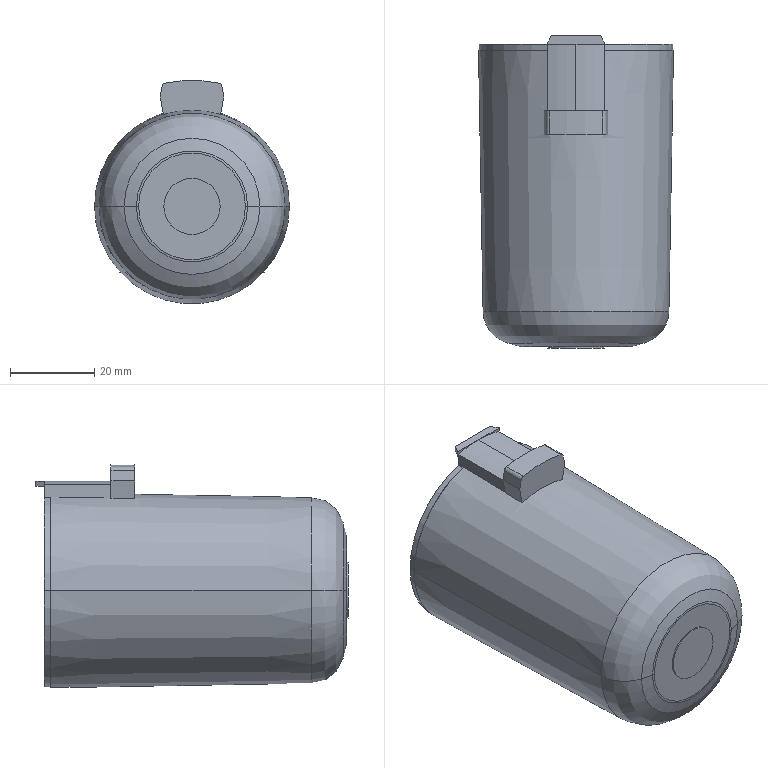Part | SolidWorks | features BaseBody 1 | 1 solid | 36 faces | box 46.4 x 74.3 x 53.2 mm | volume 114523 mm3 | plane 18 | cylinder 10 | torus 4 | cone 4 | commonest cylinder face diameters 46 x3 2 x2 13.4 x2 51.98 x2 60 x1
STEP:
#1=CARTESIAN_POINT('',(6.7,-103.95,0.));
#2=VERTEX_POINT('',#1);
#3=CARTESIAN_POINT('',(-6.7,-103.95,0.));
#4=VERTEX_POINT('',#3);
#5=CARTESIAN_POINT('',(0.,-103.95,0.));
#6=DIRECTION('',(0.,-1.,0.));
#7=DIRECTION('',(1.,0.,0.));
#8=AXIS2_PLACEMENT_3D('',#5,#6,#7);
#9=CIRCLE('',#8,6.7);
#10=EDGE_CURVE('',#2,#4,#9,.T.);
#11=ORIENTED_EDGE('',*,*,#10,.T.);
#12=CARTESIAN_POINT('',(-6.7,-104.3,0.));
#13=VERTEX_POINT('',#12);
#14=CARTESIAN_POINT('',(-6.7,-104.3,0.));
#15=DIRECTION('',(0.,-1.,0.));
#16=VECTOR('',#15,1000.);
#17=LINE('',#14,#16);
#18=EDGE_CURVE('',#4,#13,#17,.T.);
#19=ORIENTED_EDGE('',*,*,#18,.T.);
#20=CARTESIAN_POINT('',(6.7,-104.3,0.));
#21=VERTEX_POINT('',#20);
#22=CARTESIAN_POINT('',(0.,-104.3,0.));
#23=DIRECTION('',(0.,-1.,0.));
#24=DIRECTION('',(1.,0.,0.));
#25=AXIS2_PLACEMENT_3D('',#22,#23,#24);
#26=CIRCLE('',#25,6.7);
#27=EDGE_CURVE('',#21,#13,#26,.T.);
#28=ORIENTED_EDGE('',*,*,#27,.F.);
#29=CARTESIAN_POINT('',(6.7,-104.3,0.));
#30=DIRECTION('',(0.,-1.,0.));
#31=VECTOR('',#30,1000.);
#32=LINE('',#29,#31);
#33=EDGE_CURVE('',#2,#21,#32,.T.);
#34=ORIENTED_EDGE('',*,*,#33,.F.);
#35=EDGE_LOOP('',(#11,#19,#28,#34));
#36=FACE_OUTER_BOUND('',#35,.T.);
#37=CARTESIAN_POINT('',(0.,-104.3,0.));
#38=DIRECTION('',(0.,-1.,0.));
#39=DIRECTION('',(1.,0.,0.));
#40=AXIS2_PLACEMENT_3D('',#37,#38,#39);
#41=CYLINDRICAL_SURFACE('',#40,6.7);
#42=ADVANCED_FACE('',(#36),#41,.T.);
#43=CARTESIAN_POINT('',(13.254,-103.882,0.));
#44=VERTEX_POINT('',#43);
#45=CARTESIAN_POINT('',(-13.254,-103.882,0.));
#46=VERTEX_POINT('',#45);
#47=CARTESIAN_POINT('',(0.,-103.882,0.));
#48=DIRECTION('',(0.,-1.,0.));
#49=DIRECTION('',(1.,0.,0.));
#50=AXIS2_PLACEMENT_3D('',#47,#48,#49);
#51=CIRCLE('',#50,13.254);
#52=EDGE_CURVE('',#44,#46,#51,.T.);
#53=ORIENTED_EDGE('',*,*,#52,.T.);
#54=CARTESIAN_POINT('',(-12.737,-103.95,0.));
#55=VERTEX_POINT('',#54);
#56=CARTESIAN_POINT('',(-12.737,-101.95,0.));
#57=DIRECTION('',(0.,0.,1.));
#58=DIRECTION('',(1.,0.,0.));
#59=AXIS2_PLACEMENT_3D('',#56,#57,#58);
#60=CIRCLE('',#59,2.);
#61=EDGE_CURVE('',#46,#55,#60,.T.);
#62=ORIENTED_EDGE('',*,*,#61,.T.);
#63=CARTESIAN_POINT('',(12.737,-103.95,0.));
#64=VERTEX_POINT('',#63);
#65=CARTESIAN_POINT('',(0.,-103.95,0.));
#66=DIRECTION('',(0.,-1.,0.));
#67=DIRECTION('',(1.,0.,0.));
#68=AXIS2_PLACEMENT_3D('',#65,#66,#67);
#69=CIRCLE('',#68,12.737);
#70=EDGE_CURVE('',#64,#55,#69,.T.);
#71=ORIENTED_EDGE('',*,*,#70,.F.);
#72=CARTESIAN_POINT('',(12.737,-101.95,0.));
#73=DIRECTION('',(0.,0.,-1.));
#74=DIRECTION('',(-1.,0.,0.));
#75=AXIS2_PLACEMENT_3D('',#72,#73,#74);
#76=CIRCLE('',#75,2.);
#77=EDGE_CURVE('',#44,#64,#76,.T.);
#78=ORIENTED_EDGE('',*,*,#77,.F.);
#79=EDGE_LOOP('',(#53,#62,#71,#78));
#80=FACE_OUTER_BOUND('',#79,.T.);
#81=CARTESIAN_POINT('',(0.,-101.95,0.));
#82=DIRECTION('',(0.,-1.,0.));
#83=DIRECTION('',(1.,0.,0.));
#84=AXIS2_PLACEMENT_3D('',#81,#82,#83);
#85=TOROIDAL_SURFACE('',#84,12.737,2.);
#86=ADVANCED_FACE('',(#80),#85,.T.);
#87=ORIENTED_EDGE('',*,*,#52,.F.);
#88=CARTESIAN_POINT('',(16.19,-103.095,0.));
#89=VERTEX_POINT('',#88);
#90=CARTESIAN_POINT('',(16.19,-103.095,0.));
#91=DIRECTION('',(0.9659,0.2588,0.));
#92=VECTOR('',#91,1000.);
#93=LINE('',#90,#92);
#94=EDGE_CURVE('',#44,#89,#93,.T.);
#95=ORIENTED_EDGE('',*,*,#94,.T.);
#96=CARTESIAN_POINT('',(-16.19,-103.095,0.));
#97=VERTEX_POINT('',#96);
#98=CARTESIAN_POINT('',(0.,-103.095,0.));
#99=DIRECTION('',(0.,-1.,0.));
#100=DIRECTION('',(1.,0.,0.));
#101=AXIS2_PLACEMENT_3D('',#98,#99,#100);
#102=CIRCLE('',#101,16.19);
#103=EDGE_CURVE('',#89,#97,#102,.T.);
#104=ORIENTED_EDGE('',*,*,#103,.T.);
#105=CARTESIAN_POINT('',(-16.19,-103.095,0.));
#106=DIRECTION('',(-0.9659,0.2588,0.));
#107=VECTOR('',#106,1000.);
#108=LINE('',#105,#107);
#109=EDGE_CURVE('',#46,#97,#108,.T.);
#110=ORIENTED_EDGE('',*,*,#109,.F.);
#111=EDGE_LOOP('',(#87,#95,#104,#110));
#112=FACE_OUTER_BOUND('',#111,.T.);
#113=CARTESIAN_POINT('',(0.,-103.095,0.));
#114=DIRECTION('',(0.,1.,0.));
#115=DIRECTION('',(-1.,0.,0.));
#116=AXIS2_PLACEMENT_3D('',#113,#114,#115);
#117=CONICAL_SURFACE('',#116,16.19,1.309);
#118=ADVANCED_FACE('',(#112),#117,.T.);
#119=CARTESIAN_POINT('',(22.119,-95.507,0.));
#120=VERTEX_POINT('',#119);
#121=CARTESIAN_POINT('',(-22.119,-95.507,0.));
#122=VERTEX_POINT('',#121);
#123=CARTESIAN_POINT('',(0.,-95.507,0.));
#124=DIRECTION('',(0.,-1.,0.));
#125=DIRECTION('',(1.,0.,0.));
#126=AXIS2_PLACEMENT_3D('',#123,#124,#125);
#127=CIRCLE('',#126,22.119);
#128=EDGE_CURVE('',#120,#122,#127,.T.);
#129=ORIENTED_EDGE('',*,*,#128,.T.);
#130=CARTESIAN_POINT('',(-14.12,-95.368,0.));
#131=DIRECTION('',(0.,0.,1.));
#132=DIRECTION('',(1.,0.,0.));
#133=AXIS2_PLACEMENT_3D('',#130,#131,#132);
#134=CIRCLE('',#133,8.);
#135=EDGE_CURVE('',#122,#97,#134,.T.);
#136=ORIENTED_EDGE('',*,*,#135,.T.);
#137=ORIENTED_EDGE('',*,*,#103,.F.);
#138=CARTESIAN_POINT('',(14.12,-95.368,0.));
#139=DIRECTION('',(0.,0.,-1.));
#140=DIRECTION('',(-1.,0.,0.));
#141=AXIS2_PLACEMENT_3D('',#138,#139,#140);
#142=CIRCLE('',#141,8.);
#143=EDGE_CURVE('',#120,#89,#142,.T.);
#144=ORIENTED_EDGE('',*,*,#143,.F.);
#145=EDGE_LOOP('',(#129,#136,#137,#144));
#146=FACE_OUTER_BOUND('',#145,.T.);
#147=CARTESIAN_POINT('',(0.,-95.368,0.));
#148=DIRECTION('',(0.,-1.,0.));
#149=DIRECTION('',(1.,0.,0.));
#150=AXIS2_PLACEMENT_3D('',#147,#148,#149);
#151=TOROIDAL_SURFACE('',#150,14.12,8.);
#152=ADVANCED_FACE('',(#146),#151,.T.);
#153=ORIENTED_EDGE('',*,*,#128,.F.);
#154=CARTESIAN_POINT('',(23.2,-33.55,0.));
#155=VERTEX_POINT('',#154);
#156=CARTESIAN_POINT('',(23.2,-33.55,0.));
#157=DIRECTION('',(0.01745,0.9998,0.));
#158=VECTOR('',#157,1000.);
#159=LINE('',#156,#158);
#160=EDGE_CURVE('',#120,#155,#159,.T.);
#161=ORIENTED_EDGE('',*,*,#160,.T.);
#162=CARTESIAN_POINT('',(6.7,-33.55,22.211));
#163=VERTEX_POINT('',#162);
#164=CARTESIAN_POINT('',(0.,-33.55,0.));
#165=DIRECTION('',(0.,-1.,0.));
#166=DIRECTION('',(-0.2888,0.,0.9574));
#167=AXIS2_PLACEMENT_3D('',#164,#165,#166);
#168=CIRCLE('',#167,23.2);
#169=EDGE_CURVE('',#155,#163,#168,.T.);
#170=ORIENTED_EDGE('',*,*,#169,.T.);
#171=CARTESIAN_POINT('',(6.7,-47.86,21.95));
#172=VERTEX_POINT('',#171);
#173=CARTESIAN_POINT('',(6.7,-33.55,22.211));
#174=CARTESIAN_POINT('',(6.7,-38.32,22.125));
#175=CARTESIAN_POINT('',(6.7,-43.09,22.038));
#176=CARTESIAN_POINT('',(6.7,-47.86,21.95));
#177=B_SPLINE_CURVE_WITH_KNOTS('',3,(#173,#174,#175,#176),.UNSPECIFIED.,.F.,.F.,(4,4),(20.424,34.736),.UNSPECIFIED.);
#178=EDGE_CURVE('',#163,#172,#177,.T.);
#179=ORIENTED_EDGE('',*,*,#178,.T.);
#180=CARTESIAN_POINT('',(6.8,-47.86,21.92));
#181=VERTEX_POINT('',#180);
#182=CARTESIAN_POINT('',(0.,-47.86,0.));
#183=DIRECTION('',(0.,1.,0.));
#184=DIRECTION('',(0.2919,0.,0.9564));
#185=AXIS2_PLACEMENT_3D('',#182,#183,#184);
#186=CIRCLE('',#185,22.95);
#187=EDGE_CURVE('',#172,#181,#186,.T.);
#188=ORIENTED_EDGE('',*,*,#187,.T.);
#189=CARTESIAN_POINT('',(6.782,-53.5,21.822));
#190=VERTEX_POINT('',#189);
#191=CARTESIAN_POINT('',(6.782,-53.5,21.822));
#192=CARTESIAN_POINT('',(6.788,-51.62,21.855));
#193=CARTESIAN_POINT('',(6.794,-49.74,21.887));
#194=CARTESIAN_POINT('',(6.8,-47.86,21.92));
#195=B_SPLINE_CURVE_WITH_KNOTS('',3,(#191,#192,#193,#194),.UNSPECIFIED.,.F.,.F.,(4,4),(0.0002,5.641),.UNSPECIFIED.);
#196=EDGE_CURVE('',#190,#181,#195,.T.);
#197=ORIENTED_EDGE('',*,*,#196,.F.);
#198=CARTESIAN_POINT('',(-6.782,-53.5,21.822));
#199=VERTEX_POINT('',#198);
#200=CARTESIAN_POINT('',(0.,-53.5,0.));
#201=DIRECTION('',(0.,1.,0.));
#202=DIRECTION('',(-0.2968,0.,0.9549));
#203=AXIS2_PLACEMENT_3D('',#200,#201,#202);
#204=CIRCLE('',#203,22.852);
#205=EDGE_CURVE('',#199,#190,#204,.T.);
#206=ORIENTED_EDGE('',*,*,#205,.F.);
#207=CARTESIAN_POINT('',(-6.8,-47.86,21.92));
#208=VERTEX_POINT('',#207);
#209=CARTESIAN_POINT('',(-6.8,-47.86,21.92));
#210=CARTESIAN_POINT('',(-6.794,-49.74,21.887));
#211=CARTESIAN_POINT('',(-6.788,-51.62,21.855));
#212=CARTESIAN_POINT('',(-6.782,-53.5,21.822));
#213=B_SPLINE_CURVE_WITH_KNOTS('',3,(#209,#210,#211,#212),.UNSPECIFIED.,.F.,.F.,(4,4),(0.0002,5.641),.UNSPECIFIED.);
#214=EDGE_CURVE('',#208,#199,#213,.T.);
#215=ORIENTED_EDGE('',*,*,#214,.F.);
#216=CARTESIAN_POINT('',(-6.7,-47.86,21.95));
#217=VERTEX_POINT('',#216);
#218=CARTESIAN_POINT('',(0.,-47.86,0.));
#219=DIRECTION('',(0.,1.,0.));
#220=DIRECTION('',(-0.2963,0.,0.9551));
#221=AXIS2_PLACEMENT_3D('',#218,#219,#220);
#222=CIRCLE('',#221,22.95);
#223=EDGE_CURVE('',#208,#217,#222,.T.);
#224=ORIENTED_EDGE('',*,*,#223,.T.);
#225=CARTESIAN_POINT('',(-6.7,-33.55,22.211));
#226=VERTEX_POINT('',#225);
#227=CARTESIAN_POINT('',(-6.7,-47.86,21.95));
#228=CARTESIAN_POINT('',(-6.7,-43.09,22.038));
#229=CARTESIAN_POINT('',(-6.7,-38.32,22.125));
#230=CARTESIAN_POINT('',(-6.7,-33.55,22.211));
#231=B_SPLINE_CURVE_WITH_KNOTS('',3,(#227,#228,#229,#230),.UNSPECIFIED.,.F.,.F.,(4,4),(26.064,40.377),.UNSPECIFIED.);
#232=EDGE_CURVE('',#217,#226,#231,.T.);
#233=ORIENTED_EDGE('',*,*,#232,.T.);
#234=CARTESIAN_POINT('',(-23.2,-33.55,0.));
#235=VERTEX_POINT('',#234);
#236=CARTESIAN_POINT('',(0.,-33.55,0.));
#237=DIRECTION('',(0.,-1.,0.));
#238=DIRECTION('',(-0.2888,0.,0.9574));
#239=AXIS2_PLACEMENT_3D('',#236,#237,#238);
#240=CIRCLE('',#239,23.2);
#241=EDGE_CURVE('',#226,#235,#240,.T.);
#242=ORIENTED_EDGE('',*,*,#241,.T.);
#243=CARTESIAN_POINT('',(-23.2,-33.55,0.));
#244=DIRECTION('',(-0.01745,0.9998,0.));
#245=VECTOR('',#244,1000.);
#246=LINE('',#243,#245);
#247=EDGE_CURVE('',#122,#235,#246,.T.);
#248=ORIENTED_EDGE('',*,*,#247,.F.);
#249=EDGE_LOOP('',(#153,#161,#170,#179,#188,#197,#206,#215,#224,#233,#242,#248));
#250=FACE_OUTER_BOUND('',#249,.T.);
#251=CARTESIAN_POINT('',(0.,-33.55,0.));
#252=DIRECTION('',(0.,1.,0.));
#253=DIRECTION('',(-1.,0.,0.));
#254=AXIS2_PLACEMENT_3D('',#251,#252,#253);
#255=CONICAL_SURFACE('',#254,23.2,0.01745);
#256=ADVANCED_FACE('',(#250),#255,.T.);
#257=CARTESIAN_POINT('',(0.,-47.86,25.99));
#258=VERTEX_POINT('',#257);
#259=CARTESIAN_POINT('',(-6.7,-47.86,25.112));
#260=VERTEX_POINT('',#259);
#261=CARTESIAN_POINT('',(0.,-47.86,0.));
#262=DIRECTION('',(0.,-1.,0.));
#263=DIRECTION('',(0.2578,0.,0.9662));
#264=AXIS2_PLACEMENT_3D('',#261,#262,#263);
#265=CIRCLE('',#264,25.99);
#266=EDGE_CURVE('',#258,#260,#265,.T.);
#267=ORIENTED_EDGE('',*,*,#266,.F.);
#268=CARTESIAN_POINT('',(0.,-32.,25.99));
#269=VERTEX_POINT('',#268);
#270=CARTESIAN_POINT('',(0.,-53.5,25.99));
#271=DIRECTION('',(0.,1.,0.));
#272=VECTOR('',#271,1000.);
#273=LINE('',#270,#272);
#274=EDGE_CURVE('',#258,#269,#273,.T.);
#275=ORIENTED_EDGE('',*,*,#274,.T.);
#276=CARTESIAN_POINT('',(-6.7,-32.,25.112));
#277=VERTEX_POINT('',#276);
#278=CARTESIAN_POINT('',(0.,-32.,0.));
#279=DIRECTION('',(0.,1.,0.));
#280=DIRECTION('',(-0.2578,0.,0.9662));
#281=AXIS2_PLACEMENT_3D('',#278,#279,#280);
#282=CIRCLE('',#281,25.99);
#283=EDGE_CURVE('',#277,#269,#282,.T.);
#284=ORIENTED_EDGE('',*,*,#283,.F.);
#285=CARTESIAN_POINT('',(-6.7,-47.86,25.112));
#286=DIRECTION('',(0.,1.,0.));
#287=VECTOR('',#286,1000.);
#288=LINE('',#285,#287);
#289=EDGE_CURVE('',#260,#277,#288,.T.);
#290=ORIENTED_EDGE('',*,*,#289,.F.);
#291=EDGE_LOOP('',(#267,#275,#284,#290));
#292=FACE_OUTER_BOUND('',#291,.T.);
#293=CARTESIAN_POINT('',(0.,-53.5,0.));
#294=DIRECTION('',(0.,1.,0.));
#295=DIRECTION('',(0.,0.,1.));
#296=AXIS2_PLACEMENT_3D('',#293,#294,#295);
#297=CYLINDRICAL_SURFACE('',#296,25.99);
#298=ADVANCED_FACE('',(#292),#297,.T.);
#299=CARTESIAN_POINT('',(-6.7,-32.,22.002));
#300=VERTEX_POINT('',#299);
#301=CARTESIAN_POINT('',(-23.,-32.,0.));
#302=VERTEX_POINT('',#301);
#303=CARTESIAN_POINT('',(0.,-32.,0.));
#304=DIRECTION('',(0.,-1.,0.));
#305=DIRECTION('',(-0.2913,0.,0.9566));
#306=AXIS2_PLACEMENT_3D('',#303,#304,#305);
#307=CIRCLE('',#306,23.);
#308=EDGE_CURVE('',#300,#302,#307,.T.);
#309=ORIENTED_EDGE('',*,*,#308,.T.);
#310=CARTESIAN_POINT('',(-23.,-33.55,0.));
#311=VERTEX_POINT('',#310);
#312=CARTESIAN_POINT('',(-23.,-104.3,0.));
#313=DIRECTION('',(0.,-1.,0.));
#314=VECTOR('',#313,1000.);
#315=LINE('',#312,#314);
#316=EDGE_CURVE('',#302,#311,#315,.T.);
#317=ORIENTED_EDGE('',*,*,#316,.T.);
#318=CARTESIAN_POINT('',(-6.7,-33.55,22.002));
#319=VERTEX_POINT('',#318);
#320=CARTESIAN_POINT('',(0.,-33.55,0.));
#321=DIRECTION('',(0.,-1.,0.));
#322=DIRECTION('',(-0.2913,0.,0.9566));
#323=AXIS2_PLACEMENT_3D('',#320,#321,#322);
#324=CIRCLE('',#323,23.);
#325=EDGE_CURVE('',#319,#311,#324,.T.);
#326=ORIENTED_EDGE('',*,*,#325,.F.);
#327=CARTESIAN_POINT('',(-6.7,-33.55,22.002));
#328=DIRECTION('',(0.,1.,0.));
#329=VECTOR('',#328,1000.);
#330=LINE('',#327,#329);
#331=EDGE_CURVE('',#319,#300,#330,.T.);
#332=ORIENTED_EDGE('',*,*,#331,.T.);
#333=EDGE_LOOP('',(#309,#317,#326,#332));
#334=FACE_OUTER_BOUND('',#333,.T.);
#335=CARTESIAN_POINT('',(0.,-104.3,0.));
#336=DIRECTION('',(0.,-1.,0.));
#337=DIRECTION('',(1.,0.,0.));
#338=AXIS2_PLACEMENT_3D('',#335,#336,#337);
#339=CYLINDRICAL_SURFACE('',#338,23.);
#340=ADVANCED_FACE('',(#334),#339,.T.);
#341=ORIENTED_EDGE('',*,*,#316,.F.);
#342=CARTESIAN_POINT('',(23.,-32.,0.));
#343=VERTEX_POINT('',#342);
#344=CARTESIAN_POINT('',(0.,-32.,0.));
#345=DIRECTION('',(0.,-1.,0.));
#346=DIRECTION('',(-0.2913,0.,0.9566));
#347=AXIS2_PLACEMENT_3D('',#344,#345,#346);
#348=CIRCLE('',#347,23.);
#349=EDGE_CURVE('',#302,#343,#348,.T.);
#350=ORIENTED_EDGE('',*,*,#349,.T.);
#351=CARTESIAN_POINT('',(23.,-33.55,0.));
#352=VERTEX_POINT('',#351);
#353=CARTESIAN_POINT('',(23.,-104.3,0.));
#354=DIRECTION('',(0.,-1.,0.));
#355=VECTOR('',#354,1000.);
#356=LINE('',#353,#355);
#357=EDGE_CURVE('',#343,#352,#356,.T.);
#358=ORIENTED_EDGE('',*,*,#357,.T.);
#359=CARTESIAN_POINT('',(0.,-33.55,0.));
#360=DIRECTION('',(0.,-1.,0.));
#361=DIRECTION('',(-0.2913,0.,0.9566));
#362=AXIS2_PLACEMENT_3D('',#359,#360,#361);
#363=CIRCLE('',#362,23.);
#364=EDGE_CURVE('',#311,#352,#363,.T.);
#365=ORIENTED_EDGE('',*,*,#364,.F.);
#366=EDGE_LOOP('',(#341,#350,#358,#365));
#367=FACE_OUTER_BOUND('',#366,.T.);
#368=CARTESIAN_POINT('',(0.,-104.3,0.));
#369=DIRECTION('',(0.,-1.,0.));
#370=DIRECTION('',(1.,0.,0.));
#371=AXIS2_PLACEMENT_3D('',#368,#369,#370);
#372=CYLINDRICAL_SURFACE('',#371,23.);
#373=ADVANCED_FACE('',(#367),#372,.T.);
#374=ORIENTED_EDGE('',*,*,#308,.F.);
#375=CARTESIAN_POINT('',(-6.7,-32.,24.8));
#376=VERTEX_POINT('',#375);
#377=CARTESIAN_POINT('',(-6.7,-32.,22.002));
#378=DIRECTION('',(0.,0.,1.));
#379=VECTOR('',#378,1000.);
#380=LINE('',#377,#379);
#381=EDGE_CURVE('',#300,#376,#380,.T.);
#382=ORIENTED_EDGE('',*,*,#381,.T.);
#383=CARTESIAN_POINT('',(6.7,-32.,24.8));
#384=VERTEX_POINT('',#383);
#385=CARTESIAN_POINT('',(-6.7,-32.,24.8));
#386=DIRECTION('',(1.,0.,0.));
#387=VECTOR('',#386,1000.);
#388=LINE('',#385,#387);
#389=EDGE_CURVE('',#376,#384,#388,.T.);
#390=ORIENTED_EDGE('',*,*,#389,.T.);
#391=CARTESIAN_POINT('',(6.7,-32.,22.002));
#392=VERTEX_POINT('',#391);
#393=CARTESIAN_POINT('',(6.7,-32.,24.8));
#394=DIRECTION('',(0.,0.,-1.));
#395=VECTOR('',#394,1000.);
#396=LINE('',#393,#395);
#397=EDGE_CURVE('',#384,#392,#396,.T.);
#398=ORIENTED_EDGE('',*,*,#397,.T.);
#399=CARTESIAN_POINT('',(0.,-32.,0.));
#400=DIRECTION('',(0.,-1.,0.));
#401=DIRECTION('',(-0.2913,0.,0.9566));
#402=AXIS2_PLACEMENT_3D('',#399,#400,#401);
#403=CIRCLE('',#402,23.);
#404=EDGE_CURVE('',#343,#392,#403,.T.);
#405=ORIENTED_EDGE('',*,*,#404,.F.);
#406=ORIENTED_EDGE('',*,*,#349,.F.);
#407=EDGE_LOOP('',(#374,#382,#390,#398,#405,#406));
#408=FACE_OUTER_BOUND('',#407,.T.);
#409=CARTESIAN_POINT('',(0.,-32.,0.));
#410=DIRECTION('',(0.,-1.,0.));
#411=DIRECTION('',(1.,0.,0.));
#412=AXIS2_PLACEMENT_3D('',#409,#410,#411);
#413=PLANE('',#412);
#414=ADVANCED_FACE('',(#408),#413,.F.);
#415=ORIENTED_EDGE('',*,*,#357,.F.);
#416=ORIENTED_EDGE('',*,*,#404,.T.);
#417=CARTESIAN_POINT('',(6.7,-33.55,22.002));
#418=VERTEX_POINT('',#417);
#419=CARTESIAN_POINT('',(6.7,-32.,22.002));
#420=DIRECTION('',(0.,-1.,0.));
#421=VECTOR('',#420,1000.);
#422=LINE('',#419,#421);
#423=EDGE_CURVE('',#392,#418,#422,.T.);
#424=ORIENTED_EDGE('',*,*,#423,.T.);
#425=CARTESIAN_POINT('',(0.,-33.55,0.));
#426=DIRECTION('',(0.,-1.,0.));
#427=DIRECTION('',(-0.2913,0.,0.9566));
#428=AXIS2_PLACEMENT_3D('',#425,#426,#427);
#429=CIRCLE('',#428,23.);
#430=EDGE_CURVE('',#352,#418,#429,.T.);
#431=ORIENTED_EDGE('',*,*,#430,.F.);
#432=EDGE_LOOP('',(#415,#416,#424,#431));
#433=FACE_OUTER_BOUND('',#432,.T.);
#434=CARTESIAN_POINT('',(0.,-104.3,0.));
#435=DIRECTION('',(0.,-1.,0.));
#436=DIRECTION('',(1.,0.,0.));
#437=AXIS2_PLACEMENT_3D('',#434,#435,#436);
#438=CYLINDRICAL_SURFACE('',#437,23.);
#439=ADVANCED_FACE('',(#433),#438,.T.);
#440=CARTESIAN_POINT('',(-6.7,-47.86,25.112));
#441=DIRECTION('',(0.,0.,-1.));
#442=VECTOR('',#441,1000.);
#443=LINE('',#440,#442);
#444=EDGE_CURVE('',#260,#217,#443,.T.);
#445=ORIENTED_EDGE('',*,*,#444,.F.);
#446=ORIENTED_EDGE('',*,*,#289,.T.);
#447=CARTESIAN_POINT('',(-6.7,-32.,24.8));
#448=DIRECTION('',(0.,0.,1.));
#449=VECTOR('',#448,1000.);
#450=LINE('',#447,#449);
#451=EDGE_CURVE('',#376,#277,#450,.T.);
#452=ORIENTED_EDGE('',*,*,#451,.F.);
#453=ORIENTED_EDGE('',*,*,#381,.F.);
#454=ORIENTED_EDGE('',*,*,#331,.F.);
#455=CARTESIAN_POINT('',(-6.7,-33.55,22.211));
#456=DIRECTION('',(0.,0.,-1.));
#457=VECTOR('',#456,1000.);
#458=LINE('',#455,#457);
#459=EDGE_CURVE('',#226,#319,#458,.T.);
#460=ORIENTED_EDGE('',*,*,#459,.F.);
#461=ORIENTED_EDGE('',*,*,#232,.F.);
#462=EDGE_LOOP('',(#445,#446,#452,#453,#454,#460,#461));
#463=FACE_OUTER_BOUND('',#462,.T.);
#464=CARTESIAN_POINT('',(-6.7,-53.5,18.844));
#465=DIRECTION('',(-1.,0.,0.));
#466=DIRECTION('',(0.,0.,1.));
#467=AXIS2_PLACEMENT_3D('',#464,#465,#466);
#468=PLANE('',#467);
#469=ADVANCED_FACE('',(#463),#468,.T.);
#470=CARTESIAN_POINT('',(-5.845,-30.,24.8));
#471=VERTEX_POINT('',#470);
#472=CARTESIAN_POINT('',(-7.,-32.,24.8));
#473=VERTEX_POINT('',#472);
#474=CARTESIAN_POINT('',(-5.845,-30.,24.8));
#475=DIRECTION('',(-0.5,-0.866,0.));
#476=VECTOR('',#475,1000.);
#477=LINE('',#474,#476);
#478=EDGE_CURVE('',#471,#473,#477,.T.);
#479=ORIENTED_EDGE('',*,*,#478,.F.);
#480=CARTESIAN_POINT('',(5.845,-30.,24.8));
#481=VERTEX_POINT('',#480);
#482=CARTESIAN_POINT('',(5.845,-30.,24.8));
#483=DIRECTION('',(-1.,0.,0.));
#484=VECTOR('',#483,1000.);
#485=LINE('',#482,#484);
#486=EDGE_CURVE('',#481,#471,#485,.T.);
#487=ORIENTED_EDGE('',*,*,#486,.F.);
#488=CARTESIAN_POINT('',(7.,-32.,24.8));
#489=VERTEX_POINT('',#488);
#490=CARTESIAN_POINT('',(7.,-32.,24.8));
#491=DIRECTION('',(-0.5,0.866,0.));
#492=VECTOR('',#491,1000.);
#493=LINE('',#490,#492);
#494=EDGE_CURVE('',#489,#481,#493,.T.);
#495=ORIENTED_EDGE('',*,*,#494,.F.);
#496=CARTESIAN_POINT('',(6.7,-32.,24.8));
#497=DIRECTION('',(1.,0.,0.));
#498=VECTOR('',#497,1000.);
#499=LINE('',#496,#498);
#500=EDGE_CURVE('',#384,#489,#499,.T.);
#501=ORIENTED_EDGE('',*,*,#500,.F.);
#502=ORIENTED_EDGE('',*,*,#389,.F.);
#503=CARTESIAN_POINT('',(-7.,-32.,24.8));
#504=DIRECTION('',(1.,0.,0.));
#505=VECTOR('',#504,1000.);
#506=LINE('',#503,#505);
#507=EDGE_CURVE('',#473,#376,#506,.T.);
#508=ORIENTED_EDGE('',*,*,#507,.F.);
#509=EDGE_LOOP('',(#479,#487,#495,#501,#502,#508));
#510=FACE_OUTER_BOUND('',#509,.T.);
#511=CARTESIAN_POINT('',(0.,0.,24.8));
#512=DIRECTION('',(0.,0.,1.));
#513=DIRECTION('',(1.,0.,0.));
#514=AXIS2_PLACEMENT_3D('',#511,#512,#513);
#515=PLANE('',#514);
#516=ADVANCED_FACE('',(#510),#515,.F.);
#517=CARTESIAN_POINT('',(6.7,-47.86,25.112));
#518=VERTEX_POINT('',#517);
#519=CARTESIAN_POINT('',(6.7,-47.86,21.95));
#520=DIRECTION('',(0.,0.,1.));
#521=VECTOR('',#520,1000.);
#522=LINE('',#519,#521);
#523=EDGE_CURVE('',#172,#518,#522,.T.);
#524=ORIENTED_EDGE('',*,*,#523,.F.);
#525=ORIENTED_EDGE('',*,*,#178,.F.);
#526=CARTESIAN_POINT('',(6.7,-33.55,22.002));
#527=DIRECTION('',(0.,0.,1.));
#528=VECTOR('',#527,1000.);
#529=LINE('',#526,#528);
#530=EDGE_CURVE('',#418,#163,#529,.T.);
#531=ORIENTED_EDGE('',*,*,#530,.F.);
#532=ORIENTED_EDGE('',*,*,#423,.F.);
#533=ORIENTED_EDGE('',*,*,#397,.F.);
#534=CARTESIAN_POINT('',(6.7,-32.,25.112));
#535=VERTEX_POINT('',#534);
#536=CARTESIAN_POINT('',(6.7,-32.,25.112));
#537=DIRECTION('',(0.,0.,-1.));
#538=VECTOR('',#537,1000.);
#539=LINE('',#536,#538);
#540=EDGE_CURVE('',#535,#384,#539,.T.);
#541=ORIENTED_EDGE('',*,*,#540,.F.);
#542=CARTESIAN_POINT('',(6.7,-47.86,25.112));
#543=DIRECTION('',(0.,1.,0.));
#544=VECTOR('',#543,1000.);
#545=LINE('',#542,#544);
#546=EDGE_CURVE('',#518,#535,#545,.T.);
#547=ORIENTED_EDGE('',*,*,#546,.F.);
#548=EDGE_LOOP('',(#524,#525,#531,#532,#533,#541,#547));
#549=FACE_OUTER_BOUND('',#548,.T.);
#550=CARTESIAN_POINT('',(6.7,-53.5,25.112));
#551=DIRECTION('',(1.,0.,0.));
#552=DIRECTION('',(0.,0.,-1.));
#553=AXIS2_PLACEMENT_3D('',#550,#551,#552);
#554=PLANE('',#553);
#555=ADVANCED_FACE('',(#549),#554,.T.);
#556=ORIENTED_EDGE('',*,*,#241,.F.);
#557=ORIENTED_EDGE('',*,*,#459,.T.);
#558=ORIENTED_EDGE('',*,*,#325,.T.);
#559=ORIENTED_EDGE('',*,*,#364,.T.);
#560=ORIENTED_EDGE('',*,*,#430,.T.);
#561=ORIENTED_EDGE('',*,*,#530,.T.);
#562=ORIENTED_EDGE('',*,*,#169,.F.);
#563=CARTESIAN_POINT('',(0.,-33.55,0.));
#564=DIRECTION('',(0.,-1.,0.));
#565=DIRECTION('',(-0.2888,0.,0.9574));
#566=AXIS2_PLACEMENT_3D('',#563,#564,#565);
#567=CIRCLE('',#566,23.2);
#568=EDGE_CURVE('',#235,#155,#567,.T.);
#569=ORIENTED_EDGE('',*,*,#568,.F.);
#570=EDGE_LOOP('',(#556,#557,#558,#559,#560,#561,#562,#569));
#571=FACE_OUTER_BOUND('',#570,.T.);
#572=CARTESIAN_POINT('',(23.,-33.55,0.));
#573=DIRECTION('',(0.,-1.,0.));
#574=DIRECTION('',(1.,0.,0.));
#575=AXIS2_PLACEMENT_3D('',#572,#573,#574);
#576=PLANE('',#575);
#577=ADVANCED_FACE('',(#571),#576,.F.);
#578=ORIENTED_EDGE('',*,*,#187,.F.);
#579=ORIENTED_EDGE('',*,*,#523,.T.);
#580=CARTESIAN_POINT('',(0.,-47.86,0.));
#581=DIRECTION('',(0.,-1.,0.));
#582=DIRECTION('',(0.2578,0.,0.9662));
#583=AXIS2_PLACEMENT_3D('',#580,#581,#582);
#584=CIRCLE('',#583,25.99);
#585=EDGE_CURVE('',#518,#258,#584,.T.);
#586=ORIENTED_EDGE('',*,*,#585,.T.);
#587=ORIENTED_EDGE('',*,*,#266,.T.);
#588=ORIENTED_EDGE('',*,*,#444,.T.);
#589=ORIENTED_EDGE('',*,*,#223,.F.);
#590=CARTESIAN_POINT('',(-7.555,-47.86,26.024));
#591=VERTEX_POINT('',#590);
#592=CARTESIAN_POINT('',(-6.8,-47.86,21.92));
#593=DIRECTION('',(-0.1808,0.,0.9835));
#594=VECTOR('',#593,1000.);
#595=LINE('',#592,#594);
#596=EDGE_CURVE('',#208,#591,#595,.T.);
#597=ORIENTED_EDGE('',*,*,#596,.T.);
#598=CARTESIAN_POINT('',(-7.115,-47.86,28.518));
#599=VERTEX_POINT('',#598);
#600=CARTESIAN_POINT('',(-7.555,-47.86,26.024));
#601=DIRECTION('',(0.1736,0.,0.9848));
#602=VECTOR('',#601,1000.);
#603=LINE('',#600,#602);
#604=EDGE_CURVE('',#591,#599,#603,.T.);
#605=ORIENTED_EDGE('',*,*,#604,.T.);
#606=CARTESIAN_POINT('',(-6.342,-47.86,29.322));
#607=VERTEX_POINT('',#606);
#608=CARTESIAN_POINT('',(-6.13,-47.86,28.345));
#609=DIRECTION('',(0.,1.,0.));
#610=DIRECTION('',(-0.9848,0.,0.1736));
#611=AXIS2_PLACEMENT_3D('',#608,#609,#610);
#612=CIRCLE('',#611,1.);
#613=EDGE_CURVE('',#599,#607,#612,.T.);
#614=ORIENTED_EDGE('',*,*,#613,.T.);
#615=CARTESIAN_POINT('',(6.342,-47.86,29.322));
#616=VERTEX_POINT('',#615);
#617=CARTESIAN_POINT('',(0.,-47.86,0.));
#618=DIRECTION('',(0.,1.,0.));
#619=DIRECTION('',(-0.2114,0.,0.9774));
#620=AXIS2_PLACEMENT_3D('',#617,#618,#619);
#621=CIRCLE('',#620,30.);
#622=EDGE_CURVE('',#607,#616,#621,.T.);
#623=ORIENTED_EDGE('',*,*,#622,.T.);
#624=CARTESIAN_POINT('',(7.115,-47.86,28.518));
#625=VERTEX_POINT('',#624);
#626=CARTESIAN_POINT('',(6.13,-47.86,28.345));
#627=DIRECTION('',(0.,1.,0.));
#628=DIRECTION('',(0.2114,0.,0.9774));
#629=AXIS2_PLACEMENT_3D('',#626,#627,#628);
#630=CIRCLE('',#629,1.);
#631=EDGE_CURVE('',#616,#625,#630,.T.);
#632=ORIENTED_EDGE('',*,*,#631,.T.);
#633=CARTESIAN_POINT('',(7.555,-47.86,26.024));
#634=VERTEX_POINT('',#633);
#635=CARTESIAN_POINT('',(7.115,-47.86,28.518));
#636=DIRECTION('',(0.1736,0.,-0.9848));
#637=VECTOR('',#636,1000.);
#638=LINE('',#635,#637);
#639=EDGE_CURVE('',#625,#634,#638,.T.);
#640=ORIENTED_EDGE('',*,*,#639,.T.);
#641=CARTESIAN_POINT('',(7.555,-47.86,26.024));
#642=DIRECTION('',(-0.1808,0.,-0.9835));
#643=VECTOR('',#642,1000.);
#644=LINE('',#641,#643);
#645=EDGE_CURVE('',#634,#181,#644,.T.);
#646=ORIENTED_EDGE('',*,*,#645,.T.);
#647=EDGE_LOOP('',(#578,#579,#586,#587,#588,#589,#597,#605,#614,#623,#632,#640,#646));
#648=FACE_OUTER_BOUND('',#647,.T.);
#649=CARTESIAN_POINT('',(-6.13,-47.86,28.345));
#650=DIRECTION('',(0.,1.,0.));
#651=DIRECTION('',(0.,0.,1.));
#652=AXIS2_PLACEMENT_3D('',#649,#650,#651);
#653=PLANE('',#652);
#654=ADVANCED_FACE('',(#648),#653,.T.);
#655=ORIENTED_EDGE('',*,*,#274,.F.);
#656=ORIENTED_EDGE('',*,*,#585,.F.);
#657=ORIENTED_EDGE('',*,*,#546,.T.);
#658=CARTESIAN_POINT('',(0.,-32.,0.));
#659=DIRECTION('',(0.,1.,0.));
#660=DIRECTION('',(-0.2578,0.,0.9662));
#661=AXIS2_PLACEMENT_3D('',#658,#659,#660);
#662=CIRCLE('',#661,25.99);
#663=EDGE_CURVE('',#269,#535,#662,.T.);
#664=ORIENTED_EDGE('',*,*,#663,.F.);
#665=EDGE_LOOP('',(#655,#656,#657,#664));
#666=FACE_OUTER_BOUND('',#665,.T.);
#667=CARTESIAN_POINT('',(0.,-53.5,0.));
#668=DIRECTION('',(0.,1.,0.));
#669=DIRECTION('',(0.,0.,1.));
#670=AXIS2_PLACEMENT_3D('',#667,#668,#669);
#671=CYLINDRICAL_SURFACE('',#670,25.99);
#672=ADVANCED_FACE('',(#666),#671,.T.);
#673=ORIENTED_EDGE('',*,*,#283,.T.);
#674=ORIENTED_EDGE('',*,*,#663,.T.);
#675=ORIENTED_EDGE('',*,*,#540,.T.);
#676=ORIENTED_EDGE('',*,*,#500,.T.);
#677=CARTESIAN_POINT('',(7.,-32.,26.));
#678=VERTEX_POINT('',#677);
#679=CARTESIAN_POINT('',(7.,-32.,24.8));
#680=DIRECTION('',(0.,0.,1.));
#681=VECTOR('',#680,1000.);
#682=LINE('',#679,#681);
#683=EDGE_CURVE('',#489,#678,#682,.T.);
#684=ORIENTED_EDGE('',*,*,#683,.T.);
#685=CARTESIAN_POINT('',(-7.,-32.,26.));
#686=VERTEX_POINT('',#685);
#687=CARTESIAN_POINT('',(-7.,-32.,26.));
#688=DIRECTION('',(1.,0.,0.));
#689=VECTOR('',#688,1000.);
#690=LINE('',#687,#689);
#691=EDGE_CURVE('',#686,#678,#690,.T.);
#692=ORIENTED_EDGE('',*,*,#691,.F.);
#693=CARTESIAN_POINT('',(-7.,-32.,24.8));
#694=DIRECTION('',(0.,0.,1.));
#695=VECTOR('',#694,1000.);
#696=LINE('',#693,#695);
#697=EDGE_CURVE('',#473,#686,#696,.T.);
#698=ORIENTED_EDGE('',*,*,#697,.F.);
#699=ORIENTED_EDGE('',*,*,#507,.T.);
#700=ORIENTED_EDGE('',*,*,#451,.T.);
#701=EDGE_LOOP('',(#673,#674,#675,#676,#684,#692,#698,#699,#700));
#702=FACE_OUTER_BOUND('',#701,.T.);
#703=CARTESIAN_POINT('',(-7.,-32.,24.8));
#704=DIRECTION('',(0.,-1.,0.));
#705=DIRECTION('',(0.,0.,-1.));
#706=AXIS2_PLACEMENT_3D('',#703,#704,#705);
#707=PLANE('',#706);
#708=ADVANCED_FACE('',(#702),#707,.T.);
#709=ORIENTED_EDGE('',*,*,#160,.F.);
#710=CARTESIAN_POINT('',(0.,-95.507,0.));
#711=DIRECTION('',(0.,-1.,0.));
#712=DIRECTION('',(1.,0.,0.));
#713=AXIS2_PLACEMENT_3D('',#710,#711,#712);
#714=CIRCLE('',#713,22.119);
#715=EDGE_CURVE('',#122,#120,#714,.T.);
#716=ORIENTED_EDGE('',*,*,#715,.F.);
#717=ORIENTED_EDGE('',*,*,#247,.T.);
#718=ORIENTED_EDGE('',*,*,#568,.T.);
#719=EDGE_LOOP('',(#709,#716,#717,#718));
#720=FACE_OUTER_BOUND('',#719,.T.);
#721=CARTESIAN_POINT('',(0.,-33.55,0.));
#722=DIRECTION('',(0.,1.,0.));
#723=DIRECTION('',(-1.,0.,0.));
#724=AXIS2_PLACEMENT_3D('',#721,#722,#723);
#725=CONICAL_SURFACE('',#724,23.2,0.01745);
#726=ADVANCED_FACE('',(#720),#725,.T.);
#727=CARTESIAN_POINT('',(-5.845,-30.,26.));
#728=VERTEX_POINT('',#727);
#729=CARTESIAN_POINT('',(-5.845,-30.,26.));
#730=DIRECTION('',(-0.5,-0.866,0.));
#731=VECTOR('',#730,1000.);
#732=LINE('',#729,#731);
#733=EDGE_CURVE('',#728,#686,#732,.T.);
#734=ORIENTED_EDGE('',*,*,#733,.F.);
#735=CARTESIAN_POINT('',(-5.845,-30.,24.8));
#736=DIRECTION('',(0.,0.,1.));
#737=VECTOR('',#736,1000.);
#738=LINE('',#735,#737);
#739=EDGE_CURVE('',#471,#728,#738,.T.);
#740=ORIENTED_EDGE('',*,*,#739,.F.);
#741=ORIENTED_EDGE('',*,*,#478,.T.);
#742=ORIENTED_EDGE('',*,*,#697,.T.);
#743=EDGE_LOOP('',(#734,#740,#741,#742));
#744=FACE_OUTER_BOUND('',#743,.T.);
#745=CARTESIAN_POINT('',(-5.845,-30.,24.8));
#746=DIRECTION('',(-0.866,0.5,0.));
#747=DIRECTION('',(-0.5,-0.866,0.));
#748=AXIS2_PLACEMENT_3D('',#745,#746,#747);
#749=PLANE('',#748);
#750=ADVANCED_FACE('',(#744),#749,.T.);
#751=CARTESIAN_POINT('',(5.845,-30.,26.));
#752=VERTEX_POINT('',#751);
#753=CARTESIAN_POINT('',(5.845,-30.,26.));
#754=DIRECTION('',(-1.,0.,0.));
#755=VECTOR('',#754,1000.);
#756=LINE('',#753,#755);
#757=EDGE_CURVE('',#752,#728,#756,.T.);
#758=ORIENTED_EDGE('',*,*,#757,.F.);
#759=CARTESIAN_POINT('',(5.845,-30.,24.8));
#760=DIRECTION('',(0.,0.,1.));
#761=VECTOR('',#760,1000.);
#762=LINE('',#759,#761);
#763=EDGE_CURVE('',#481,#752,#762,.T.);
#764=ORIENTED_EDGE('',*,*,#763,.F.);
#765=ORIENTED_EDGE('',*,*,#486,.T.);
#766=ORIENTED_EDGE('',*,*,#739,.T.);
#767=EDGE_LOOP('',(#758,#764,#765,#766));
#768=FACE_OUTER_BOUND('',#767,.T.);
#769=CARTESIAN_POINT('',(5.845,-30.,24.8));
#770=DIRECTION('',(0.,1.,0.));
#771=DIRECTION('',(0.,0.,1.));
#772=AXIS2_PLACEMENT_3D('',#769,#770,#771);
#773=PLANE('',#772);
#774=ADVANCED_FACE('',(#768),#773,.T.);
#775=CARTESIAN_POINT('',(7.,-32.,26.));
#776=DIRECTION('',(-0.5,0.866,0.));
#777=VECTOR('',#776,1000.);
#778=LINE('',#775,#777);
#779=EDGE_CURVE('',#678,#752,#778,.T.);
#780=ORIENTED_EDGE('',*,*,#779,.F.);
#781=ORIENTED_EDGE('',*,*,#683,.F.);
#782=ORIENTED_EDGE('',*,*,#494,.T.);
#783=ORIENTED_EDGE('',*,*,#763,.T.);
#784=EDGE_LOOP('',(#780,#781,#782,#783));
#785=FACE_OUTER_BOUND('',#784,.T.);
#786=CARTESIAN_POINT('',(7.,-32.,24.8));
#787=DIRECTION('',(0.866,0.5,0.));
#788=DIRECTION('',(-0.5,0.866,0.));
#789=AXIS2_PLACEMENT_3D('',#786,#787,#788);
#790=PLANE('',#789);
#791=ADVANCED_FACE('',(#785),#790,.T.);
#792=ORIENTED_EDGE('',*,*,#596,.F.);
#793=ORIENTED_EDGE('',*,*,#214,.T.);
#794=CARTESIAN_POINT('',(-7.555,-53.5,26.024));
#795=VERTEX_POINT('',#794);
#796=CARTESIAN_POINT('',(-6.782,-53.5,21.822));
#797=DIRECTION('',(-0.1808,0.,0.9835));
#798=VECTOR('',#797,1000.);
#799=LINE('',#796,#798);
#800=EDGE_CURVE('',#199,#795,#799,.T.);
#801=ORIENTED_EDGE('',*,*,#800,.T.);
#802=CARTESIAN_POINT('',(-7.555,-47.86,26.024));
#803=DIRECTION('',(0.,-1.,0.));
#804=VECTOR('',#803,1000.);
#805=LINE('',#802,#804);
#806=EDGE_CURVE('',#591,#795,#805,.T.);
#807=ORIENTED_EDGE('',*,*,#806,.F.);
#808=EDGE_LOOP('',(#792,#793,#801,#807));
#809=FACE_OUTER_BOUND('',#808,.T.);
#810=CARTESIAN_POINT('',(-6.7,-47.86,21.375));
#811=DIRECTION('',(0.9835,0.,0.1808));
#812=DIRECTION('',(0.1808,0.,-0.9835));
#813=AXIS2_PLACEMENT_3D('',#810,#811,#812);
#814=PLANE('',#813);
#815=ADVANCED_FACE('',(#809),#814,.F.);
#816=CARTESIAN_POINT('',(-7.115,-53.5,28.518));
#817=VERTEX_POINT('',#816);
#818=CARTESIAN_POINT('',(-7.555,-53.5,26.024));
#819=DIRECTION('',(0.1736,0.,0.9848));
#820=VECTOR('',#819,1000.);
#821=LINE('',#818,#820);
#822=EDGE_CURVE('',#795,#817,#821,.T.);
#823=ORIENTED_EDGE('',*,*,#822,.T.);
#824=CARTESIAN_POINT('',(-7.115,-47.86,28.518));
#825=DIRECTION('',(0.,-1.,0.));
#826=VECTOR('',#825,1000.);
#827=LINE('',#824,#826);
#828=EDGE_CURVE('',#599,#817,#827,.T.);
#829=ORIENTED_EDGE('',*,*,#828,.F.);
#830=ORIENTED_EDGE('',*,*,#604,.F.);
#831=ORIENTED_EDGE('',*,*,#806,.T.);
#832=EDGE_LOOP('',(#823,#829,#830,#831));
#833=FACE_OUTER_BOUND('',#832,.T.);
#834=CARTESIAN_POINT('',(-7.555,-47.86,26.024));
#835=DIRECTION('',(0.9848,0.,-0.1736));
#836=DIRECTION('',(-0.1736,0.,-0.9848));
#837=AXIS2_PLACEMENT_3D('',#834,#835,#836);
#838=PLANE('',#837);
#839=ADVANCED_FACE('',(#833),#838,.F.);
#840=CARTESIAN_POINT('',(-6.342,-53.5,29.322));
#841=VERTEX_POINT('',#840);
#842=CARTESIAN_POINT('',(-6.13,-53.5,28.345));
#843=DIRECTION('',(0.,1.,0.));
#844=DIRECTION('',(-0.9848,0.,0.1736));
#845=AXIS2_PLACEMENT_3D('',#842,#843,#844);
#846=CIRCLE('',#845,1.);
#847=EDGE_CURVE('',#817,#841,#846,.T.);
#848=ORIENTED_EDGE('',*,*,#847,.T.);
#849=CARTESIAN_POINT('',(-6.342,-47.86,29.322));
#850=DIRECTION('',(0.,-1.,0.));
#851=VECTOR('',#850,1000.);
#852=LINE('',#849,#851);
#853=EDGE_CURVE('',#607,#841,#852,.T.);
#854=ORIENTED_EDGE('',*,*,#853,.F.);
#855=ORIENTED_EDGE('',*,*,#613,.F.);
#856=ORIENTED_EDGE('',*,*,#828,.T.);
#857=EDGE_LOOP('',(#848,#854,#855,#856));
#858=FACE_OUTER_BOUND('',#857,.T.);
#859=CARTESIAN_POINT('',(-6.13,-47.86,28.345));
#860=DIRECTION('',(0.,-1.,0.));
#861=DIRECTION('',(0.,0.,-1.));
#862=AXIS2_PLACEMENT_3D('',#859,#860,#861);
#863=CYLINDRICAL_SURFACE('',#862,1.);
#864=ADVANCED_FACE('',(#858),#863,.T.);
#865=CARTESIAN_POINT('',(6.342,-53.5,29.322));
#866=VERTEX_POINT('',#865);
#867=CARTESIAN_POINT('',(0.,-53.5,0.));
#868=DIRECTION('',(0.,1.,0.));
#869=DIRECTION('',(-0.2114,0.,0.9774));
#870=AXIS2_PLACEMENT_3D('',#867,#868,#869);
#871=CIRCLE('',#870,30.);
#872=EDGE_CURVE('',#841,#866,#871,.T.);
#873=ORIENTED_EDGE('',*,*,#872,.T.);
#874=CARTESIAN_POINT('',(6.342,-47.86,29.322));
#875=DIRECTION('',(0.,-1.,0.));
#876=VECTOR('',#875,1000.);
#877=LINE('',#874,#876);
#878=EDGE_CURVE('',#616,#866,#877,.T.);
#879=ORIENTED_EDGE('',*,*,#878,.F.);
#880=ORIENTED_EDGE('',*,*,#622,.F.);
#881=ORIENTED_EDGE('',*,*,#853,.T.);
#882=EDGE_LOOP('',(#873,#879,#880,#881));
#883=FACE_OUTER_BOUND('',#882,.T.);
#884=CARTESIAN_POINT('',(0.,-47.86,0.));
#885=DIRECTION('',(0.,-1.,0.));
#886=DIRECTION('',(0.,0.,-1.));
#887=AXIS2_PLACEMENT_3D('',#884,#885,#886);
#888=CYLINDRICAL_SURFACE('',#887,30.);
#889=ADVANCED_FACE('',(#883),#888,.T.);
#890=CARTESIAN_POINT('',(7.115,-53.5,28.518));
#891=VERTEX_POINT('',#890);
#892=CARTESIAN_POINT('',(6.13,-53.5,28.345));
#893=DIRECTION('',(0.,1.,0.));
#894=DIRECTION('',(0.2114,0.,0.9774));
#895=AXIS2_PLACEMENT_3D('',#892,#893,#894);
#896=CIRCLE('',#895,1.);
#897=EDGE_CURVE('',#866,#891,#896,.T.);
#898=ORIENTED_EDGE('',*,*,#897,.T.);
#899=CARTESIAN_POINT('',(7.115,-47.86,28.518));
#900=DIRECTION('',(0.,-1.,0.));
#901=VECTOR('',#900,1000.);
#902=LINE('',#899,#901);
#903=EDGE_CURVE('',#625,#891,#902,.T.);
#904=ORIENTED_EDGE('',*,*,#903,.F.);
#905=ORIENTED_EDGE('',*,*,#631,.F.);
#906=ORIENTED_EDGE('',*,*,#878,.T.);
#907=EDGE_LOOP('',(#898,#904,#905,#906));
#908=FACE_OUTER_BOUND('',#907,.T.);
#909=CARTESIAN_POINT('',(6.13,-47.86,28.345));
#910=DIRECTION('',(0.,-1.,0.));
#911=DIRECTION('',(0.,0.,-1.));
#912=AXIS2_PLACEMENT_3D('',#909,#910,#911);
#913=CYLINDRICAL_SURFACE('',#912,1.);
#914=ADVANCED_FACE('',(#908),#913,.T.);
#915=CARTESIAN_POINT('',(7.555,-53.5,26.024));
#916=VERTEX_POINT('',#915);
#917=CARTESIAN_POINT('',(7.115,-53.5,28.518));
#918=DIRECTION('',(0.1736,0.,-0.9848));
#919=VECTOR('',#918,1000.);
#920=LINE('',#917,#919);
#921=EDGE_CURVE('',#891,#916,#920,.T.);
#922=ORIENTED_EDGE('',*,*,#921,.T.);
#923=CARTESIAN_POINT('',(7.555,-47.86,26.024));
#924=DIRECTION('',(0.,-1.,0.));
#925=VECTOR('',#924,1000.);
#926=LINE('',#923,#925);
#927=EDGE_CURVE('',#634,#916,#926,.T.);
#928=ORIENTED_EDGE('',*,*,#927,.F.);
#929=ORIENTED_EDGE('',*,*,#639,.F.);
#930=ORIENTED_EDGE('',*,*,#903,.T.);
#931=EDGE_LOOP('',(#922,#928,#929,#930));
#932=FACE_OUTER_BOUND('',#931,.T.);
#933=CARTESIAN_POINT('',(7.115,-47.86,28.518));
#934=DIRECTION('',(-0.9848,0.,-0.1736));
#935=DIRECTION('',(-0.1736,0.,0.9848));
#936=AXIS2_PLACEMENT_3D('',#933,#934,#935);
#937=PLANE('',#936);
#938=ADVANCED_FACE('',(#932),#937,.F.);
#939=CARTESIAN_POINT('',(7.555,-53.5,26.024));
#940=DIRECTION('',(-0.1808,0.,-0.9835));
#941=VECTOR('',#940,1000.);
#942=LINE('',#939,#941);
#943=EDGE_CURVE('',#916,#190,#942,.T.);
#944=ORIENTED_EDGE('',*,*,#943,.T.);
#945=ORIENTED_EDGE('',*,*,#196,.T.);
#946=ORIENTED_EDGE('',*,*,#645,.F.);
#947=ORIENTED_EDGE('',*,*,#927,.T.);
#948=EDGE_LOOP('',(#944,#945,#946,#947));
#949=FACE_OUTER_BOUND('',#948,.T.);
#950=CARTESIAN_POINT('',(7.555,-47.86,26.024));
#951=DIRECTION('',(-0.9835,0.,0.1808));
#952=DIRECTION('',(0.1808,0.,0.9835));
#953=AXIS2_PLACEMENT_3D('',#950,#951,#952);
#954=PLANE('',#953);
#955=ADVANCED_FACE('',(#949),#954,.F.);
#956=ORIENTED_EDGE('',*,*,#733,.T.);
#957=ORIENTED_EDGE('',*,*,#691,.T.);
#958=ORIENTED_EDGE('',*,*,#779,.T.);
#959=ORIENTED_EDGE('',*,*,#757,.T.);
#960=EDGE_LOOP('',(#956,#957,#958,#959));
#961=FACE_OUTER_BOUND('',#960,.T.);
#962=CARTESIAN_POINT('',(0.,0.,26.));
#963=DIRECTION('',(0.,0.,1.));
#964=DIRECTION('',(1.,0.,0.));
#965=AXIS2_PLACEMENT_3D('',#962,#963,#964);
#966=PLANE('',#965);
#967=ADVANCED_FACE('',(#961),#966,.T.);
#968=ORIENTED_EDGE('',*,*,#135,.F.);
#969=ORIENTED_EDGE('',*,*,#715,.T.);
#970=ORIENTED_EDGE('',*,*,#143,.T.);
#971=CARTESIAN_POINT('',(0.,-103.095,0.));
#972=DIRECTION('',(0.,-1.,0.));
#973=DIRECTION('',(1.,0.,0.));
#974=AXIS2_PLACEMENT_3D('',#971,#972,#973);
#975=CIRCLE('',#974,16.19);
#976=EDGE_CURVE('',#97,#89,#975,.T.);
#977=ORIENTED_EDGE('',*,*,#976,.F.);
#978=EDGE_LOOP('',(#968,#969,#970,#977));
#979=FACE_OUTER_BOUND('',#978,.T.);
#980=CARTESIAN_POINT('',(0.,-95.368,0.));
#981=DIRECTION('',(0.,-1.,0.));
#982=DIRECTION('',(1.,0.,0.));
#983=AXIS2_PLACEMENT_3D('',#980,#981,#982);
#984=TOROIDAL_SURFACE('',#983,14.12,8.);
#985=ADVANCED_FACE('',(#979),#984,.T.);
#986=ORIENTED_EDGE('',*,*,#205,.T.);
#987=ORIENTED_EDGE('',*,*,#943,.F.);
#988=ORIENTED_EDGE('',*,*,#921,.F.);
#989=ORIENTED_EDGE('',*,*,#897,.F.);
#990=ORIENTED_EDGE('',*,*,#872,.F.);
#991=ORIENTED_EDGE('',*,*,#847,.F.);
#992=ORIENTED_EDGE('',*,*,#822,.F.);
#993=ORIENTED_EDGE('',*,*,#800,.F.);
#994=EDGE_LOOP('',(#986,#987,#988,#989,#990,#991,#992,#993));
#995=FACE_OUTER_BOUND('',#994,.T.);
#996=CARTESIAN_POINT('',(0.,-53.5,0.));
#997=DIRECTION('',(0.,1.,0.));
#998=DIRECTION('',(0.,0.,1.));
#999=AXIS2_PLACEMENT_3D('',#996,#997,#998);
#1000=PLANE('',#999);
#1001=ADVANCED_FACE('',(#995),#1000,.F.);
#1002=ORIENTED_EDGE('',*,*,#94,.F.);
#1003=CARTESIAN_POINT('',(0.,-103.882,0.));
#1004=DIRECTION('',(0.,-1.,0.));
#1005=DIRECTION('',(1.,0.,0.));
#1006=AXIS2_PLACEMENT_3D('',#1003,#1004,#1005);
#1007=CIRCLE('',#1006,13.254);
#1008=EDGE_CURVE('',#46,#44,#1007,.T.);
#1009=ORIENTED_EDGE('',*,*,#1008,.F.);
#1010=ORIENTED_EDGE('',*,*,#109,.T.);
#1011=ORIENTED_EDGE('',*,*,#976,.T.);
#1012=EDGE_LOOP('',(#1002,#1009,#1010,#1011));
#1013=FACE_OUTER_BOUND('',#1012,.T.);
#1014=CARTESIAN_POINT('',(0.,-103.095,0.));
#1015=DIRECTION('',(0.,1.,0.));
#1016=DIRECTION('',(-1.,0.,0.));
#1017=AXIS2_PLACEMENT_3D('',#1014,#1015,#1016);
#1018=CONICAL_SURFACE('',#1017,16.19,1.309);
#1019=ADVANCED_FACE('',(#1013),#1018,.T.);
#1020=ORIENTED_EDGE('',*,*,#61,.F.);
#1021=ORIENTED_EDGE('',*,*,#1008,.T.);
#1022=ORIENTED_EDGE('',*,*,#77,.T.);
#1023=CARTESIAN_POINT('',(0.,-103.95,0.));
#1024=DIRECTION('',(0.,-1.,0.));
#1025=DIRECTION('',(1.,0.,0.));
#1026=AXIS2_PLACEMENT_3D('',#1023,#1024,#1025);
#1027=CIRCLE('',#1026,12.737);
#1028=EDGE_CURVE('',#55,#64,#1027,.T.);
#1029=ORIENTED_EDGE('',*,*,#1028,.F.);
#1030=EDGE_LOOP('',(#1020,#1021,#1022,#1029));
#1031=FACE_OUTER_BOUND('',#1030,.T.);
#1032=CARTESIAN_POINT('',(0.,-101.95,0.));
#1033=DIRECTION('',(0.,-1.,0.));
#1034=DIRECTION('',(1.,0.,0.));
#1035=AXIS2_PLACEMENT_3D('',#1032,#1033,#1034);
#1036=TOROIDAL_SURFACE('',#1035,12.737,2.);
#1037=ADVANCED_FACE('',(#1031),#1036,.T.);
#1038=ORIENTED_EDGE('',*,*,#10,.F.);
#1039=CARTESIAN_POINT('',(0.,-103.95,0.));
#1040=DIRECTION('',(0.,-1.,0.));
#1041=DIRECTION('',(1.,0.,0.));
#1042=AXIS2_PLACEMENT_3D('',#1039,#1040,#1041);
#1043=CIRCLE('',#1042,6.7);
#1044=EDGE_CURVE('',#4,#2,#1043,.T.);
#1045=ORIENTED_EDGE('',*,*,#1044,.F.);
#1046=EDGE_LOOP('',(#1038,#1045));
#1047=FACE_BOUND('',#1046,.T.);
#1048=ORIENTED_EDGE('',*,*,#70,.T.);
#1049=ORIENTED_EDGE('',*,*,#1028,.T.);
#1050=EDGE_LOOP('',(#1048,#1049));
#1051=FACE_OUTER_BOUND('',#1050,.T.);
#1052=CARTESIAN_POINT('',(12.737,-103.95,0.));
#1053=DIRECTION('',(0.,1.,0.));
#1054=DIRECTION('',(-1.,0.,0.));
#1055=AXIS2_PLACEMENT_3D('',#1052,#1053,#1054);
#1056=PLANE('',#1055);
#1057=ADVANCED_FACE('',(#1047,#1051),#1056,.F.);
#1058=ORIENTED_EDGE('',*,*,#18,.F.);
#1059=ORIENTED_EDGE('',*,*,#1044,.T.);
#1060=ORIENTED_EDGE('',*,*,#33,.T.);
#1061=CARTESIAN_POINT('',(0.,-104.3,0.));
#1062=DIRECTION('',(0.,-1.,0.));
#1063=DIRECTION('',(1.,0.,0.));
#1064=AXIS2_PLACEMENT_3D('',#1061,#1062,#1063);
#1065=CIRCLE('',#1064,6.7);
#1066=EDGE_CURVE('',#13,#21,#1065,.T.);
#1067=ORIENTED_EDGE('',*,*,#1066,.F.);
#1068=EDGE_LOOP('',(#1058,#1059,#1060,#1067));
#1069=FACE_OUTER_BOUND('',#1068,.T.);
#1070=CARTESIAN_POINT('',(0.,-104.3,0.));
#1071=DIRECTION('',(0.,-1.,0.));
#1072=DIRECTION('',(1.,0.,0.));
#1073=AXIS2_PLACEMENT_3D('',#1070,#1071,#1072);
#1074=CYLINDRICAL_SURFACE('',#1073,6.7);
#1075=ADVANCED_FACE('',(#1069),#1074,.T.);
#1076=ORIENTED_EDGE('',*,*,#27,.T.);
#1077=ORIENTED_EDGE('',*,*,#1066,.T.);
#1078=EDGE_LOOP('',(#1076,#1077));
#1079=FACE_OUTER_BOUND('',#1078,.T.);
#1080=CARTESIAN_POINT('',(6.7,-104.3,0.));
#1081=DIRECTION('',(0.,1.,0.));
#1082=DIRECTION('',(-1.,0.,0.));
#1083=AXIS2_PLACEMENT_3D('',#1080,#1081,#1082);
#1084=PLANE('',#1083);
#1085=ADVANCED_FACE('',(#1079),#1084,.F.);
#1086=CLOSED_SHELL('',(#42,#86,#118,#152,#256,#298,#340,#373,#414,#439,#469,#516,#555,#577,#654,#672,#708,#726,#750,#774,#791,#815,#839,#864,#889,#914,#938,#955,#967,#985,#1001,#1019,#1037,#1057,#1075,#1085));
#1087=MANIFOLD_SOLID_BREP('',#1086);
#1088=CARTESIAN_POINT('',(0.,0.,0.));
#1089=DIRECTION('',(0.,0.,1.));
#1090=DIRECTION('',(1.,0.,0.));
#1091=AXIS2_PLACEMENT_3D('',#1088,#1089,#1090);
#1092=(LENGTH_UNIT()NAMED_UNIT(*)SI_UNIT(.MILLI.,.METRE.));
#1093=UNCERTAINTY_MEASURE_WITH_UNIT(LENGTH_MEASURE(0.00001),#1092,'','');
#1094=(NAMED_UNIT(*)PLANE_ANGLE_UNIT()SI_UNIT($,.RADIAN.));
#1095=(NAMED_UNIT(*)SI_UNIT($,.STERADIAN.)SOLID_ANGLE_UNIT());
#1096=(GEOMETRIC_REPRESENTATION_CONTEXT(3)GLOBAL_UNCERTAINTY_ASSIGNED_CONTEXT((#1093))GLOBAL_UNIT_ASSIGNED_CONTEXT((#1092,#1094,#1095))REPRESENTATION_CONTEXT('',''));
#1097=ADVANCED_BREP_SHAPE_REPRESENTATION('',(#1087,#1091),#1096);